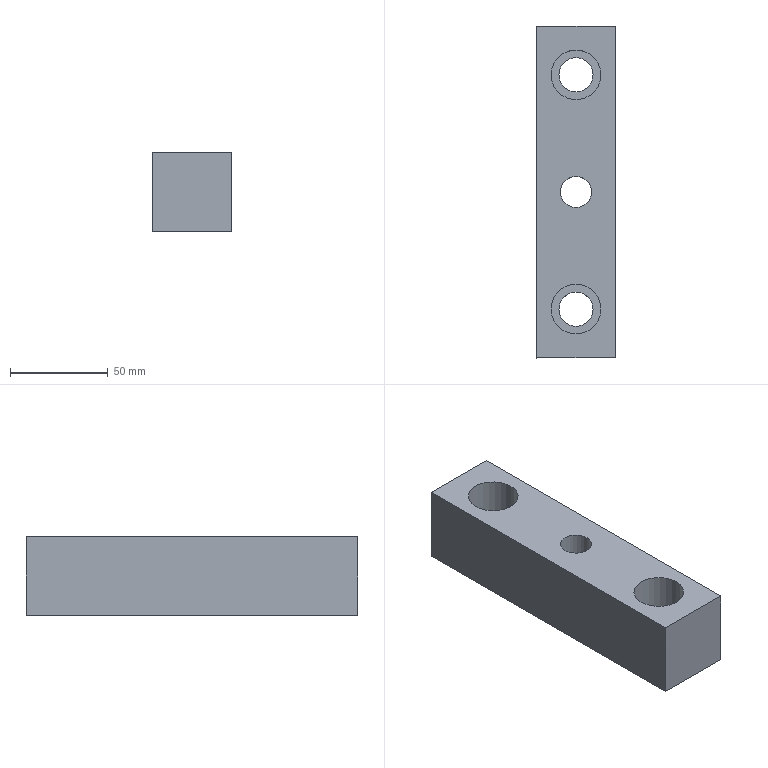Part | NX | features MAIN_BODY 2 | 1 solid | 13 faces | box 40 x 170 x 40 mm | volume 233908 mm3 | plane 8 | cylinder 5 | commonest cylinder face diameters 17.5 x2 25.5 x2 16 x1
STEP:
#1=CARTESIAN_POINT('',(1062.,380.,-260.));
#2=VERTEX_POINT('',#1);
#3=CARTESIAN_POINT('',(1070.,380.,-260.));
#4=DIRECTION('',(0.000000001,-0.00000017,-1.));
#5=DIRECTION('',(-1.,0.,-0.000000001));
#6=AXIS2_PLACEMENT_3D('',#3,#4,#5);
#7=CIRCLE('',#6,8.);
#8=EDGE_CURVE('',#2,#2,#7,.T.);
#9=ORIENTED_EDGE('',*,*,#8,.T.);
#10=EDGE_LOOP('',(#9));
#11=FACE_BOUND('',#10,.T.);
#12=CARTESIAN_POINT('',(1057.25,320.,-260.));
#13=VERTEX_POINT('',#12);
#14=CARTESIAN_POINT('',(1070.,320.,-260.));
#15=DIRECTION('',(0.000000001,-0.00000017,-1.));
#16=DIRECTION('',(-1.,0.,-0.000000001));
#17=AXIS2_PLACEMENT_3D('',#14,#15,#16);
#18=CIRCLE('',#17,12.75);
#19=EDGE_CURVE('',#13,#13,#18,.F.);
#20=ORIENTED_EDGE('',*,*,#19,.F.);
#21=EDGE_LOOP('',(#20));
#22=FACE_BOUND('',#21,.T.);
#23=CARTESIAN_POINT('',(1050.,465.,-260.));
#24=VERTEX_POINT('',#23);
#25=CARTESIAN_POINT('',(1050.,295.,-260.));
#26=VERTEX_POINT('',#25);
#27=CARTESIAN_POINT('',(1050.,672.,-260.));
#28=DIRECTION('',(-0.000000011,1.,-0.00000017));
#29=VECTOR('',#28,1000.);
#30=LINE('',#27,#29);
#31=EDGE_CURVE('',#24,#26,#30,.F.);
#32=ORIENTED_EDGE('',*,*,#31,.T.);
#33=CARTESIAN_POINT('',(1090.,295.,-260.));
#34=VERTEX_POINT('',#33);
#35=CARTESIAN_POINT('',(1090.,295.,-260.));
#36=DIRECTION('',(-1.,-0.000000011,-0.000000001));
#37=VECTOR('',#36,1000.);
#38=LINE('',#35,#37);
#39=EDGE_CURVE('',#34,#26,#38,.T.);
#40=ORIENTED_EDGE('',*,*,#39,.F.);
#41=CARTESIAN_POINT('',(1090.,465.,-260.));
#42=VERTEX_POINT('',#41);
#43=CARTESIAN_POINT('',(1090.,672.,-260.));
#44=DIRECTION('',(-0.000000011,1.,-0.00000017));
#45=VECTOR('',#44,1000.);
#46=LINE('',#43,#45);
#47=EDGE_CURVE('',#42,#34,#46,.F.);
#48=ORIENTED_EDGE('',*,*,#47,.F.);
#49=CARTESIAN_POINT('',(1090.,465.,-260.));
#50=DIRECTION('',(-1.,-0.000000011,-0.000000001));
#51=VECTOR('',#50,1000.);
#52=LINE('',#49,#51);
#53=EDGE_CURVE('',#42,#24,#52,.T.);
#54=ORIENTED_EDGE('',*,*,#53,.T.);
#55=EDGE_LOOP('',(#32,#40,#48,#54));
#56=FACE_BOUND('',#55,.T.);
#57=CARTESIAN_POINT('',(1057.25,440.,-260.));
#58=VERTEX_POINT('',#57);
#59=CARTESIAN_POINT('',(1070.,440.,-260.));
#60=DIRECTION('',(0.000000001,-0.00000017,-1.));
#61=DIRECTION('',(-1.,0.,-0.000000001));
#62=AXIS2_PLACEMENT_3D('',#59,#60,#61);
#63=CIRCLE('',#62,12.75);
#64=EDGE_CURVE('',#58,#58,#63,.F.);
#65=ORIENTED_EDGE('',*,*,#64,.F.);
#66=EDGE_LOOP('',(#65));
#67=FACE_BOUND('',#66,.T.);
#68=CARTESIAN_POINT('',(1090.,672.,-260.));
#69=DIRECTION('',(0.000000001,-0.00000017,-1.));
#70=DIRECTION('',(-1.,0.,-0.000000001));
#71=AXIS2_PLACEMENT_3D('',#68,#69,#70);
#72=PLANE('',#71);
#73=ADVANCED_FACE('',(#11,#22,#56,#67),#72,.F.);
#74=CARTESIAN_POINT('',(1078.75,440.,-300.));
#75=VERTEX_POINT('',#74);
#76=CARTESIAN_POINT('',(1070.,440.,-300.));
#77=DIRECTION('',(-0.000000001,0.00000017,1.));
#78=DIRECTION('',(1.,0.,0.000000001));
#79=AXIS2_PLACEMENT_3D('',#76,#77,#78);
#80=CIRCLE('',#79,8.75);
#81=EDGE_CURVE('',#75,#75,#80,.T.);
#82=ORIENTED_EDGE('',*,*,#81,.F.);
#83=EDGE_LOOP('',(#82));
#84=FACE_BOUND('',#83,.T.);
#85=CARTESIAN_POINT('',(1078.75,440.,-280.));
#86=VERTEX_POINT('',#85);
#87=CARTESIAN_POINT('',(1070.,440.,-280.));
#88=DIRECTION('',(-0.000000001,0.00000017,1.));
#89=DIRECTION('',(1.,0.,0.000000001));
#90=AXIS2_PLACEMENT_3D('',#87,#88,#89);
#91=CIRCLE('',#90,8.75);
#92=EDGE_CURVE('',#86,#86,#91,.F.);
#93=ORIENTED_EDGE('',*,*,#92,.F.);
#94=EDGE_LOOP('',(#93));
#95=FACE_BOUND('',#94,.T.);
#96=CARTESIAN_POINT('',(1070.,440.,-260.));
#97=DIRECTION('',(0.000000001,-0.00000017,-1.));
#98=DIRECTION('',(-1.,0.,-0.000000001));
#99=AXIS2_PLACEMENT_3D('',#96,#97,#98);
#100=CYLINDRICAL_SURFACE('',#99,8.75);
#101=ADVANCED_FACE('',(#84,#95),#100,.F.);
#102=CARTESIAN_POINT('',(1078.75,320.,-300.));
#103=VERTEX_POINT('',#102);
#104=CARTESIAN_POINT('',(1070.,320.,-300.));
#105=DIRECTION('',(-0.000000001,0.00000017,1.));
#106=DIRECTION('',(1.,0.,0.000000001));
#107=AXIS2_PLACEMENT_3D('',#104,#105,#106);
#108=CIRCLE('',#107,8.75);
#109=EDGE_CURVE('',#103,#103,#108,.T.);
#110=ORIENTED_EDGE('',*,*,#109,.F.);
#111=EDGE_LOOP('',(#110));
#112=FACE_BOUND('',#111,.T.);
#113=CARTESIAN_POINT('',(1078.75,320.,-280.));
#114=VERTEX_POINT('',#113);
#115=CARTESIAN_POINT('',(1070.,320.,-280.));
#116=DIRECTION('',(-0.000000001,0.00000017,1.));
#117=DIRECTION('',(1.,0.,0.000000001));
#118=AXIS2_PLACEMENT_3D('',#115,#116,#117);
#119=CIRCLE('',#118,8.75);
#120=EDGE_CURVE('',#114,#114,#119,.F.);
#121=ORIENTED_EDGE('',*,*,#120,.F.);
#122=EDGE_LOOP('',(#121));
#123=FACE_BOUND('',#122,.T.);
#124=CARTESIAN_POINT('',(1070.,320.,-260.));
#125=DIRECTION('',(0.000000001,-0.00000017,-1.));
#126=DIRECTION('',(-1.,0.,-0.000000001));
#127=AXIS2_PLACEMENT_3D('',#124,#125,#126);
#128=CYLINDRICAL_SURFACE('',#127,8.75);
#129=ADVANCED_FACE('',(#112,#123),#128,.F.);
#130=CARTESIAN_POINT('',(1050.,465.,-300.));
#131=VERTEX_POINT('',#130);
#132=CARTESIAN_POINT('',(1050.,465.,-209.));
#133=DIRECTION('',(-0.000000001,0.00000017,1.));
#134=VECTOR('',#133,1000.);
#135=LINE('',#132,#134);
#136=EDGE_CURVE('',#131,#24,#135,.T.);
#137=ORIENTED_EDGE('',*,*,#136,.T.);
#138=ORIENTED_EDGE('',*,*,#53,.F.);
#139=CARTESIAN_POINT('',(1090.,465.,-300.));
#140=VERTEX_POINT('',#139);
#141=CARTESIAN_POINT('',(1090.,465.,-209.));
#142=DIRECTION('',(-0.000000001,0.00000017,1.));
#143=VECTOR('',#142,1000.);
#144=LINE('',#141,#143);
#145=EDGE_CURVE('',#140,#42,#144,.T.);
#146=ORIENTED_EDGE('',*,*,#145,.F.);
#147=CARTESIAN_POINT('',(1090.,465.,-300.));
#148=DIRECTION('',(-1.,-0.000000011,-0.000000001));
#149=VECTOR('',#148,1000.);
#150=LINE('',#147,#149);
#151=EDGE_CURVE('',#140,#131,#150,.T.);
#152=ORIENTED_EDGE('',*,*,#151,.T.);
#153=EDGE_LOOP('',(#137,#138,#146,#152));
#154=FACE_BOUND('',#153,.T.);
#155=CARTESIAN_POINT('',(1090.,465.,-209.));
#156=DIRECTION('',(0.000000011,-1.,0.00000017));
#157=DIRECTION('',(1.,0.000000011,0.000000171));
#158=AXIS2_PLACEMENT_3D('',#155,#156,#157);
#159=PLANE('',#158);
#160=ADVANCED_FACE('',(#154),#159,.F.);
#161=CARTESIAN_POINT('',(1078.,380.,-300.));
#162=VERTEX_POINT('',#161);
#163=CARTESIAN_POINT('',(1070.,380.,-300.));
#164=DIRECTION('',(-0.000000001,0.00000017,1.));
#165=DIRECTION('',(1.,0.,0.000000001));
#166=AXIS2_PLACEMENT_3D('',#163,#164,#165);
#167=CIRCLE('',#166,8.);
#168=EDGE_CURVE('',#162,#162,#167,.T.);
#169=ORIENTED_EDGE('',*,*,#168,.T.);
#170=EDGE_LOOP('',(#169));
#171=FACE_BOUND('',#170,.T.);
#172=ORIENTED_EDGE('',*,*,#81,.T.);
#173=EDGE_LOOP('',(#172));
#174=FACE_BOUND('',#173,.T.);
#175=ORIENTED_EDGE('',*,*,#109,.T.);
#176=EDGE_LOOP('',(#175));
#177=FACE_BOUND('',#176,.T.);
#178=CARTESIAN_POINT('',(1050.,295.,-300.));
#179=VERTEX_POINT('',#178);
#180=CARTESIAN_POINT('',(1050.,355.,-300.));
#181=DIRECTION('',(0.000000011,-1.,0.00000017));
#182=VECTOR('',#181,1000.);
#183=LINE('',#180,#182);
#184=EDGE_CURVE('',#179,#131,#183,.F.);
#185=ORIENTED_EDGE('',*,*,#184,.T.);
#186=ORIENTED_EDGE('',*,*,#151,.F.);
#187=CARTESIAN_POINT('',(1090.,295.,-300.));
#188=VERTEX_POINT('',#187);
#189=CARTESIAN_POINT('',(1090.,355.,-300.));
#190=DIRECTION('',(0.000000011,-1.,0.00000017));
#191=VECTOR('',#190,1000.);
#192=LINE('',#189,#191);
#193=EDGE_CURVE('',#188,#140,#192,.F.);
#194=ORIENTED_EDGE('',*,*,#193,.F.);
#195=CARTESIAN_POINT('',(1090.,295.,-300.));
#196=DIRECTION('',(-1.,-0.000000011,-0.000000001));
#197=VECTOR('',#196,1000.);
#198=LINE('',#195,#197);
#199=EDGE_CURVE('',#188,#179,#198,.T.);
#200=ORIENTED_EDGE('',*,*,#199,.T.);
#201=EDGE_LOOP('',(#185,#186,#194,#200));
#202=FACE_BOUND('',#201,.T.);
#203=CARTESIAN_POINT('',(1090.,355.,-300.));
#204=DIRECTION('',(-0.000000001,0.00000017,1.));
#205=DIRECTION('',(1.,0.,0.000000001));
#206=AXIS2_PLACEMENT_3D('',#203,#204,#205);
#207=PLANE('',#206);
#208=ADVANCED_FACE('',(#171,#174,#177,#202),#207,.F.);
#209=CARTESIAN_POINT('',(1050.,295.,-209.));
#210=DIRECTION('',(0.000000001,-0.00000017,-1.));
#211=VECTOR('',#210,1000.);
#212=LINE('',#209,#211);
#213=EDGE_CURVE('',#179,#26,#212,.F.);
#214=ORIENTED_EDGE('',*,*,#213,.F.);
#215=ORIENTED_EDGE('',*,*,#199,.F.);
#216=CARTESIAN_POINT('',(1090.,295.,-209.));
#217=DIRECTION('',(0.000000001,-0.00000017,-1.));
#218=VECTOR('',#217,1000.);
#219=LINE('',#216,#218);
#220=EDGE_CURVE('',#188,#34,#219,.F.);
#221=ORIENTED_EDGE('',*,*,#220,.T.);
#222=ORIENTED_EDGE('',*,*,#39,.T.);
#223=EDGE_LOOP('',(#214,#215,#221,#222));
#224=FACE_BOUND('',#223,.T.);
#225=CARTESIAN_POINT('',(1090.,295.,-209.));
#226=DIRECTION('',(0.000000011,-1.,0.00000017));
#227=DIRECTION('',(1.,0.000000011,0.000000171));
#228=AXIS2_PLACEMENT_3D('',#225,#226,#227);
#229=PLANE('',#228);
#230=ADVANCED_FACE('',(#224),#229,.T.);
#231=ORIENTED_EDGE('',*,*,#47,.T.);
#232=ORIENTED_EDGE('',*,*,#220,.F.);
#233=ORIENTED_EDGE('',*,*,#193,.T.);
#234=ORIENTED_EDGE('',*,*,#145,.T.);
#235=EDGE_LOOP('',(#231,#232,#233,#234));
#236=FACE_BOUND('',#235,.T.);
#237=CARTESIAN_POINT('',(1090.,355.,-209.));
#238=DIRECTION('',(1.,0.000000011,0.000000001));
#239=DIRECTION('',(0.000000011,-1.,0.00000017));
#240=AXIS2_PLACEMENT_3D('',#237,#238,#239);
#241=PLANE('',#240);
#242=ADVANCED_FACE('',(#236),#241,.T.);
#243=ORIENTED_EDGE('',*,*,#31,.F.);
#244=ORIENTED_EDGE('',*,*,#136,.F.);
#245=ORIENTED_EDGE('',*,*,#184,.F.);
#246=ORIENTED_EDGE('',*,*,#213,.T.);
#247=EDGE_LOOP('',(#243,#244,#245,#246));
#248=FACE_BOUND('',#247,.T.);
#249=CARTESIAN_POINT('',(1050.,355.,-209.));
#250=DIRECTION('',(1.,0.000000011,0.000000001));
#251=DIRECTION('',(0.000000011,-1.,0.00000017));
#252=AXIS2_PLACEMENT_3D('',#249,#250,#251);
#253=PLANE('',#252);
#254=ADVANCED_FACE('',(#248),#253,.F.);
#255=CARTESIAN_POINT('',(1082.75,320.,-280.));
#256=VERTEX_POINT('',#255);
#257=CARTESIAN_POINT('',(1070.,320.,-280.));
#258=DIRECTION('',(-0.000000001,0.00000017,1.));
#259=DIRECTION('',(1.,0.,0.000000001));
#260=AXIS2_PLACEMENT_3D('',#257,#258,#259);
#261=CIRCLE('',#260,12.75);
#262=EDGE_CURVE('',#256,#256,#261,.T.);
#263=ORIENTED_EDGE('',*,*,#262,.F.);
#264=EDGE_LOOP('',(#263));
#265=FACE_BOUND('',#264,.T.);
#266=ORIENTED_EDGE('',*,*,#19,.T.);
#267=EDGE_LOOP('',(#266));
#268=FACE_BOUND('',#267,.T.);
#269=CARTESIAN_POINT('',(1070.,320.,-200.));
#270=DIRECTION('',(0.000000001,-0.00000017,-1.));
#271=DIRECTION('',(-1.,0.,-0.000000001));
#272=AXIS2_PLACEMENT_3D('',#269,#270,#271);
#273=CYLINDRICAL_SURFACE('',#272,12.75);
#274=ADVANCED_FACE('',(#265,#268),#273,.F.);
#275=ORIENTED_EDGE('',*,*,#262,.T.);
#276=EDGE_LOOP('',(#275));
#277=FACE_BOUND('',#276,.T.);
#278=ORIENTED_EDGE('',*,*,#120,.T.);
#279=EDGE_LOOP('',(#278));
#280=FACE_BOUND('',#279,.T.);
#281=CARTESIAN_POINT('',(1070.,240.,-280.));
#282=DIRECTION('',(-0.000000001,0.00000017,1.));
#283=DIRECTION('',(1.,0.,0.000000001));
#284=AXIS2_PLACEMENT_3D('',#281,#282,#283);
#285=PLANE('',#284);
#286=ADVANCED_FACE('',(#277,#280),#285,.T.);
#287=CARTESIAN_POINT('',(1082.75,440.,-280.));
#288=VERTEX_POINT('',#287);
#289=CARTESIAN_POINT('',(1070.,440.,-280.));
#290=DIRECTION('',(-0.000000001,0.00000017,1.));
#291=DIRECTION('',(1.,0.,0.000000001));
#292=AXIS2_PLACEMENT_3D('',#289,#290,#291);
#293=CIRCLE('',#292,12.75);
#294=EDGE_CURVE('',#288,#288,#293,.T.);
#295=ORIENTED_EDGE('',*,*,#294,.F.);
#296=EDGE_LOOP('',(#295));
#297=FACE_BOUND('',#296,.T.);
#298=ORIENTED_EDGE('',*,*,#64,.T.);
#299=EDGE_LOOP('',(#298));
#300=FACE_BOUND('',#299,.T.);
#301=CARTESIAN_POINT('',(1070.,440.,-200.));
#302=DIRECTION('',(0.000000001,-0.00000017,-1.));
#303=DIRECTION('',(-1.,0.,-0.000000001));
#304=AXIS2_PLACEMENT_3D('',#301,#302,#303);
#305=CYLINDRICAL_SURFACE('',#304,12.75);
#306=ADVANCED_FACE('',(#297,#300),#305,.F.);
#307=ORIENTED_EDGE('',*,*,#294,.T.);
#308=EDGE_LOOP('',(#307));
#309=FACE_BOUND('',#308,.T.);
#310=ORIENTED_EDGE('',*,*,#92,.T.);
#311=EDGE_LOOP('',(#310));
#312=FACE_BOUND('',#311,.T.);
#313=CARTESIAN_POINT('',(1070.,440.,-280.));
#314=DIRECTION('',(-0.000000001,0.00000017,1.));
#315=DIRECTION('',(1.,0.,0.000000001));
#316=AXIS2_PLACEMENT_3D('',#313,#314,#315);
#317=PLANE('',#316);
#318=ADVANCED_FACE('',(#309,#312),#317,.T.);
#319=ORIENTED_EDGE('',*,*,#168,.F.);
#320=EDGE_LOOP('',(#319));
#321=FACE_BOUND('',#320,.T.);
#322=ORIENTED_EDGE('',*,*,#8,.F.);
#323=EDGE_LOOP('',(#322));
#324=FACE_BOUND('',#323,.T.);
#325=CARTESIAN_POINT('',(1070.,380.,-360.));
#326=DIRECTION('',(-0.000000171,0.00000017,1.));
#327=DIRECTION('',(0.,1.,-0.00000017));
#328=AXIS2_PLACEMENT_3D('',#325,#326,#327);
#329=CYLINDRICAL_SURFACE('',#328,8.);
#330=ADVANCED_FACE('',(#321,#324),#329,.F.);
#331=CLOSED_SHELL('',(#73,#101,#129,#160,#208,#230,#242,#254,#274,#286,#306,#318,#330));
#332=MANIFOLD_SOLID_BREP('',#331);
#333=(LENGTH_UNIT()NAMED_UNIT(*)SI_UNIT(.MILLI.,.METRE.));
#334=UNCERTAINTY_MEASURE_WITH_UNIT(LENGTH_MEASURE(0.00001),#333,'','');
#335=(NAMED_UNIT(*)PLANE_ANGLE_UNIT()SI_UNIT($,.RADIAN.));
#336=(NAMED_UNIT(*)SI_UNIT($,.STERADIAN.)SOLID_ANGLE_UNIT());
#337=(GEOMETRIC_REPRESENTATION_CONTEXT(3)GLOBAL_UNCERTAINTY_ASSIGNED_CONTEXT((#334))GLOBAL_UNIT_ASSIGNED_CONTEXT((#333,#335,#336))REPRESENTATION_CONTEXT('',''));
#338=ADVANCED_BREP_SHAPE_REPRESENTATION('',(#332),#337);